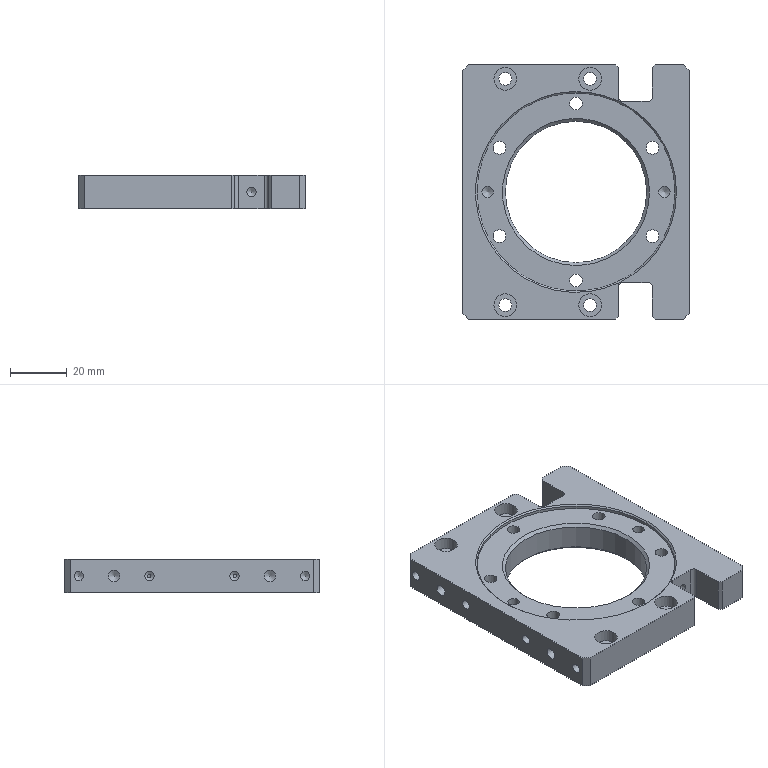Part | 1 solid | 90 faces | box 80 x 90 x 12 mm | volume 51348 mm3 | cylinder 40 | plane 33 | cone 17 | commonest cylinder face diameters 3.3 x10 4.5 x10 8 x10 3 x4 4 x4 50 x1